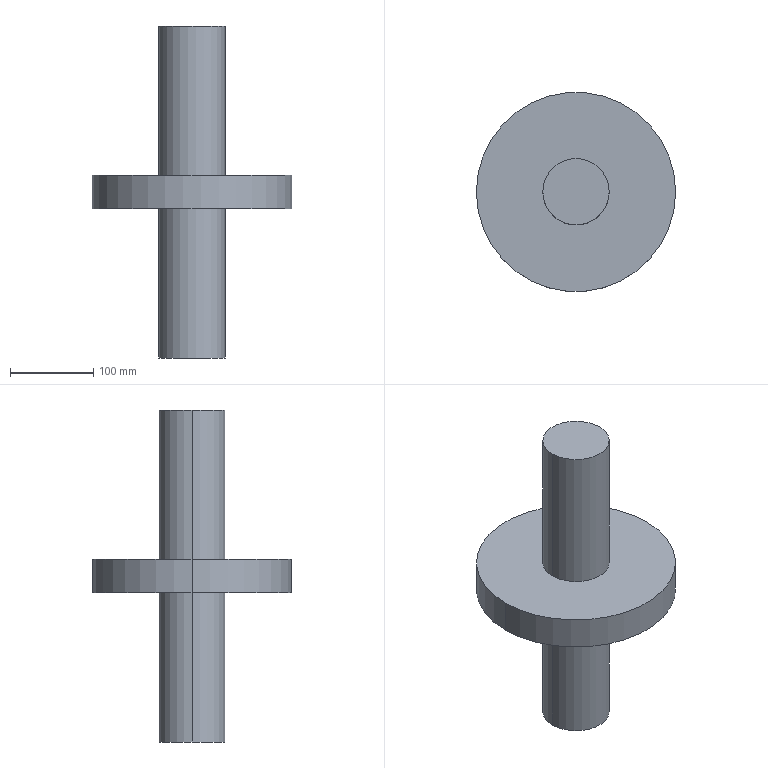Part | SolidWorks | features Extrusion 1, ICE 1 | 1 solid | 10 faces | box 240 x 240 x 400 mm | volume 3619115 mm3 | cylinder 6 | plane 4 | commonest cylinder face diameters 80 x4 240 x2
STEP:
#1=CARTESIAN_POINT('',(40.,0.,-20.));
#2=VERTEX_POINT('',#1);
#3=CARTESIAN_POINT('',(-40.,0.,-20.));
#4=VERTEX_POINT('',#3);
#5=CARTESIAN_POINT('',(0.,0.,-20.));
#6=DIRECTION('',(0.,0.,1.));
#7=DIRECTION('',(1.,0.,0.));
#8=AXIS2_PLACEMENT_3D('',#5,#6,#7);
#9=CIRCLE('',#8,40.);
#10=EDGE_CURVE('',#2,#4,#9,.T.);
#11=ORIENTED_EDGE('',*,*,#10,.F.);
#12=CARTESIAN_POINT('',(40.,0.,-200.));
#13=VERTEX_POINT('',#12);
#14=CARTESIAN_POINT('',(40.,0.,200.));
#15=DIRECTION('',(0.,0.,-1.));
#16=VECTOR('',#15,1000.);
#17=LINE('',#14,#16);
#18=EDGE_CURVE('',#2,#13,#17,.T.);
#19=ORIENTED_EDGE('',*,*,#18,.T.);
#20=CARTESIAN_POINT('',(-40.,0.,-200.));
#21=VERTEX_POINT('',#20);
#22=CARTESIAN_POINT('',(0.,0.,-200.));
#23=DIRECTION('',(0.,0.,1.));
#24=DIRECTION('',(1.,0.,0.));
#25=AXIS2_PLACEMENT_3D('',#22,#23,#24);
#26=CIRCLE('',#25,40.);
#27=EDGE_CURVE('',#13,#21,#26,.T.);
#28=ORIENTED_EDGE('',*,*,#27,.T.);
#29=CARTESIAN_POINT('',(-40.,0.,200.));
#30=DIRECTION('',(0.,0.,-1.));
#31=VECTOR('',#30,1000.);
#32=LINE('',#29,#31);
#33=EDGE_CURVE('',#4,#21,#32,.T.);
#34=ORIENTED_EDGE('',*,*,#33,.F.);
#35=EDGE_LOOP('',(#11,#19,#28,#34));
#36=FACE_OUTER_BOUND('',#35,.T.);
#37=CARTESIAN_POINT('',(0.,0.,200.));
#38=DIRECTION('',(0.,0.,-1.));
#39=DIRECTION('',(-1.,0.,0.));
#40=AXIS2_PLACEMENT_3D('',#37,#38,#39);
#41=CYLINDRICAL_SURFACE('',#40,40.);
#42=ADVANCED_FACE('',(#36),#41,.T.);
#43=CARTESIAN_POINT('',(120.,0.,20.));
#44=VERTEX_POINT('',#43);
#45=CARTESIAN_POINT('',(-120.,0.,20.));
#46=VERTEX_POINT('',#45);
#47=CARTESIAN_POINT('',(0.,0.,20.));
#48=DIRECTION('',(0.,0.,1.));
#49=DIRECTION('',(1.,0.,0.));
#50=AXIS2_PLACEMENT_3D('',#47,#48,#49);
#51=CIRCLE('',#50,120.);
#52=EDGE_CURVE('',#44,#46,#51,.T.);
#53=ORIENTED_EDGE('',*,*,#52,.F.);
#54=CARTESIAN_POINT('',(120.,0.,-20.));
#55=VERTEX_POINT('',#54);
#56=CARTESIAN_POINT('',(120.,0.,20.));
#57=DIRECTION('',(0.,0.,-1.));
#58=VECTOR('',#57,1000.);
#59=LINE('',#56,#58);
#60=EDGE_CURVE('',#44,#55,#59,.T.);
#61=ORIENTED_EDGE('',*,*,#60,.T.);
#62=CARTESIAN_POINT('',(-120.,0.,-20.));
#63=VERTEX_POINT('',#62);
#64=CARTESIAN_POINT('',(0.,0.,-20.));
#65=DIRECTION('',(0.,0.,1.));
#66=DIRECTION('',(1.,0.,0.));
#67=AXIS2_PLACEMENT_3D('',#64,#65,#66);
#68=CIRCLE('',#67,120.);
#69=EDGE_CURVE('',#55,#63,#68,.T.);
#70=ORIENTED_EDGE('',*,*,#69,.T.);
#71=CARTESIAN_POINT('',(-120.,0.,20.));
#72=DIRECTION('',(0.,0.,-1.));
#73=VECTOR('',#72,1000.);
#74=LINE('',#71,#73);
#75=EDGE_CURVE('',#46,#63,#74,.T.);
#76=ORIENTED_EDGE('',*,*,#75,.F.);
#77=EDGE_LOOP('',(#53,#61,#70,#76));
#78=FACE_OUTER_BOUND('',#77,.T.);
#79=CARTESIAN_POINT('',(0.,0.,20.));
#80=DIRECTION('',(0.,0.,-1.));
#81=DIRECTION('',(-1.,0.,0.));
#82=AXIS2_PLACEMENT_3D('',#79,#80,#81);
#83=CYLINDRICAL_SURFACE('',#82,120.);
#84=ADVANCED_FACE('',(#78),#83,.T.);
#85=CARTESIAN_POINT('',(40.,0.,200.));
#86=VERTEX_POINT('',#85);
#87=CARTESIAN_POINT('',(-40.,0.,200.));
#88=VERTEX_POINT('',#87);
#89=CARTESIAN_POINT('',(0.,0.,200.));
#90=DIRECTION('',(0.,0.,1.));
#91=DIRECTION('',(1.,0.,0.));
#92=AXIS2_PLACEMENT_3D('',#89,#90,#91);
#93=CIRCLE('',#92,40.);
#94=EDGE_CURVE('',#86,#88,#93,.T.);
#95=ORIENTED_EDGE('',*,*,#94,.F.);
#96=CARTESIAN_POINT('',(40.,0.,20.));
#97=VERTEX_POINT('',#96);
#98=CARTESIAN_POINT('',(40.,0.,200.));
#99=DIRECTION('',(0.,0.,-1.));
#100=VECTOR('',#99,1000.);
#101=LINE('',#98,#100);
#102=EDGE_CURVE('',#86,#97,#101,.T.);
#103=ORIENTED_EDGE('',*,*,#102,.T.);
#104=CARTESIAN_POINT('',(-40.,0.,20.));
#105=VERTEX_POINT('',#104);
#106=CARTESIAN_POINT('',(0.,0.,20.));
#107=DIRECTION('',(0.,0.,1.));
#108=DIRECTION('',(1.,0.,0.));
#109=AXIS2_PLACEMENT_3D('',#106,#107,#108);
#110=CIRCLE('',#109,40.);
#111=EDGE_CURVE('',#97,#105,#110,.T.);
#112=ORIENTED_EDGE('',*,*,#111,.T.);
#113=CARTESIAN_POINT('',(-40.,0.,200.));
#114=DIRECTION('',(0.,0.,-1.));
#115=VECTOR('',#114,1000.);
#116=LINE('',#113,#115);
#117=EDGE_CURVE('',#88,#105,#116,.T.);
#118=ORIENTED_EDGE('',*,*,#117,.F.);
#119=EDGE_LOOP('',(#95,#103,#112,#118));
#120=FACE_OUTER_BOUND('',#119,.T.);
#121=CARTESIAN_POINT('',(0.,0.,200.));
#122=DIRECTION('',(0.,0.,-1.));
#123=DIRECTION('',(-1.,0.,0.));
#124=AXIS2_PLACEMENT_3D('',#121,#122,#123);
#125=CYLINDRICAL_SURFACE('',#124,40.);
#126=ADVANCED_FACE('',(#120),#125,.T.);
#127=ORIENTED_EDGE('',*,*,#102,.F.);
#128=CARTESIAN_POINT('',(0.,0.,200.));
#129=DIRECTION('',(0.,0.,1.));
#130=DIRECTION('',(1.,0.,0.));
#131=AXIS2_PLACEMENT_3D('',#128,#129,#130);
#132=CIRCLE('',#131,40.);
#133=EDGE_CURVE('',#88,#86,#132,.T.);
#134=ORIENTED_EDGE('',*,*,#133,.F.);
#135=ORIENTED_EDGE('',*,*,#117,.T.);
#136=CARTESIAN_POINT('',(0.,0.,20.));
#137=DIRECTION('',(0.,0.,1.));
#138=DIRECTION('',(1.,0.,0.));
#139=AXIS2_PLACEMENT_3D('',#136,#137,#138);
#140=CIRCLE('',#139,40.);
#141=EDGE_CURVE('',#105,#97,#140,.T.);
#142=ORIENTED_EDGE('',*,*,#141,.T.);
#143=EDGE_LOOP('',(#127,#134,#135,#142));
#144=FACE_OUTER_BOUND('',#143,.T.);
#145=CARTESIAN_POINT('',(0.,0.,200.));
#146=DIRECTION('',(0.,0.,-1.));
#147=DIRECTION('',(-1.,0.,0.));
#148=AXIS2_PLACEMENT_3D('',#145,#146,#147);
#149=CYLINDRICAL_SURFACE('',#148,40.);
#150=ADVANCED_FACE('',(#144),#149,.T.);
#151=ORIENTED_EDGE('',*,*,#133,.T.);
#152=ORIENTED_EDGE('',*,*,#94,.T.);
#153=EDGE_LOOP('',(#151,#152));
#154=FACE_OUTER_BOUND('',#153,.T.);
#155=CARTESIAN_POINT('',(0.,0.,200.));
#156=DIRECTION('',(0.,0.,1.));
#157=DIRECTION('',(1.,0.,0.));
#158=AXIS2_PLACEMENT_3D('',#155,#156,#157);
#159=PLANE('',#158);
#160=ADVANCED_FACE('',(#154),#159,.T.);
#161=ORIENTED_EDGE('',*,*,#60,.F.);
#162=CARTESIAN_POINT('',(0.,0.,20.));
#163=DIRECTION('',(0.,0.,1.));
#164=DIRECTION('',(1.,0.,0.));
#165=AXIS2_PLACEMENT_3D('',#162,#163,#164);
#166=CIRCLE('',#165,120.);
#167=EDGE_CURVE('',#46,#44,#166,.T.);
#168=ORIENTED_EDGE('',*,*,#167,.F.);
#169=ORIENTED_EDGE('',*,*,#75,.T.);
#170=CARTESIAN_POINT('',(0.,0.,-20.));
#171=DIRECTION('',(0.,0.,1.));
#172=DIRECTION('',(1.,0.,0.));
#173=AXIS2_PLACEMENT_3D('',#170,#171,#172);
#174=CIRCLE('',#173,120.);
#175=EDGE_CURVE('',#63,#55,#174,.T.);
#176=ORIENTED_EDGE('',*,*,#175,.T.);
#177=EDGE_LOOP('',(#161,#168,#169,#176));
#178=FACE_OUTER_BOUND('',#177,.T.);
#179=CARTESIAN_POINT('',(0.,0.,20.));
#180=DIRECTION('',(0.,0.,-1.));
#181=DIRECTION('',(-1.,0.,0.));
#182=AXIS2_PLACEMENT_3D('',#179,#180,#181);
#183=CYLINDRICAL_SURFACE('',#182,120.);
#184=ADVANCED_FACE('',(#178),#183,.T.);
#185=ORIENTED_EDGE('',*,*,#141,.F.);
#186=ORIENTED_EDGE('',*,*,#111,.F.);
#187=EDGE_LOOP('',(#185,#186));
#188=FACE_BOUND('',#187,.T.);
#189=ORIENTED_EDGE('',*,*,#167,.T.);
#190=ORIENTED_EDGE('',*,*,#52,.T.);
#191=EDGE_LOOP('',(#189,#190));
#192=FACE_OUTER_BOUND('',#191,.T.);
#193=CARTESIAN_POINT('',(0.,0.,20.));
#194=DIRECTION('',(0.,0.,1.));
#195=DIRECTION('',(1.,0.,0.));
#196=AXIS2_PLACEMENT_3D('',#193,#194,#195);
#197=PLANE('',#196);
#198=ADVANCED_FACE('',(#188,#192),#197,.T.);
#199=CARTESIAN_POINT('',(0.,0.,-20.));
#200=DIRECTION('',(0.,0.,1.));
#201=DIRECTION('',(1.,0.,0.));
#202=AXIS2_PLACEMENT_3D('',#199,#200,#201);
#203=CIRCLE('',#202,40.);
#204=EDGE_CURVE('',#4,#2,#203,.T.);
#205=ORIENTED_EDGE('',*,*,#204,.T.);
#206=ORIENTED_EDGE('',*,*,#10,.T.);
#207=EDGE_LOOP('',(#205,#206));
#208=FACE_BOUND('',#207,.T.);
#209=ORIENTED_EDGE('',*,*,#175,.F.);
#210=ORIENTED_EDGE('',*,*,#69,.F.);
#211=EDGE_LOOP('',(#209,#210));
#212=FACE_OUTER_BOUND('',#211,.T.);
#213=CARTESIAN_POINT('',(0.,0.,-20.));
#214=DIRECTION('',(0.,0.,1.));
#215=DIRECTION('',(1.,0.,0.));
#216=AXIS2_PLACEMENT_3D('',#213,#214,#215);
#217=PLANE('',#216);
#218=ADVANCED_FACE('',(#208,#212),#217,.F.);
#219=CARTESIAN_POINT('',(0.,0.,-200.));
#220=DIRECTION('',(0.,0.,1.));
#221=DIRECTION('',(1.,0.,0.));
#222=AXIS2_PLACEMENT_3D('',#219,#220,#221);
#223=CIRCLE('',#222,40.);
#224=EDGE_CURVE('',#21,#13,#223,.T.);
#225=ORIENTED_EDGE('',*,*,#224,.F.);
#226=ORIENTED_EDGE('',*,*,#27,.F.);
#227=EDGE_LOOP('',(#225,#226));
#228=FACE_OUTER_BOUND('',#227,.T.);
#229=CARTESIAN_POINT('',(0.,0.,-200.));
#230=DIRECTION('',(0.,0.,1.));
#231=DIRECTION('',(1.,0.,0.));
#232=AXIS2_PLACEMENT_3D('',#229,#230,#231);
#233=PLANE('',#232);
#234=ADVANCED_FACE('',(#228),#233,.F.);
#235=ORIENTED_EDGE('',*,*,#18,.F.);
#236=ORIENTED_EDGE('',*,*,#204,.F.);
#237=ORIENTED_EDGE('',*,*,#33,.T.);
#238=ORIENTED_EDGE('',*,*,#224,.T.);
#239=EDGE_LOOP('',(#235,#236,#237,#238));
#240=FACE_OUTER_BOUND('',#239,.T.);
#241=CARTESIAN_POINT('',(0.,0.,200.));
#242=DIRECTION('',(0.,0.,-1.));
#243=DIRECTION('',(-1.,0.,0.));
#244=AXIS2_PLACEMENT_3D('',#241,#242,#243);
#245=CYLINDRICAL_SURFACE('',#244,40.);
#246=ADVANCED_FACE('',(#240),#245,.T.);
#247=CLOSED_SHELL('',(#42,#84,#126,#150,#160,#184,#198,#218,#234,#246));
#248=MANIFOLD_SOLID_BREP('',#247);
#249=CARTESIAN_POINT('',(0.,0.,0.));
#250=DIRECTION('',(0.,0.,1.));
#251=DIRECTION('',(1.,0.,0.));
#252=AXIS2_PLACEMENT_3D('',#249,#250,#251);
#253=(LENGTH_UNIT()NAMED_UNIT(*)SI_UNIT(.MILLI.,.METRE.));
#254=UNCERTAINTY_MEASURE_WITH_UNIT(LENGTH_MEASURE(0.00001),#253,'','');
#255=(NAMED_UNIT(*)PLANE_ANGLE_UNIT()SI_UNIT($,.RADIAN.));
#256=(NAMED_UNIT(*)SI_UNIT($,.STERADIAN.)SOLID_ANGLE_UNIT());
#257=(GEOMETRIC_REPRESENTATION_CONTEXT(3)GLOBAL_UNCERTAINTY_ASSIGNED_CONTEXT((#254))GLOBAL_UNIT_ASSIGNED_CONTEXT((#253,#255,#256))REPRESENTATION_CONTEXT('',''));
#258=ADVANCED_BREP_SHAPE_REPRESENTATION('',(#248,#252),#257);